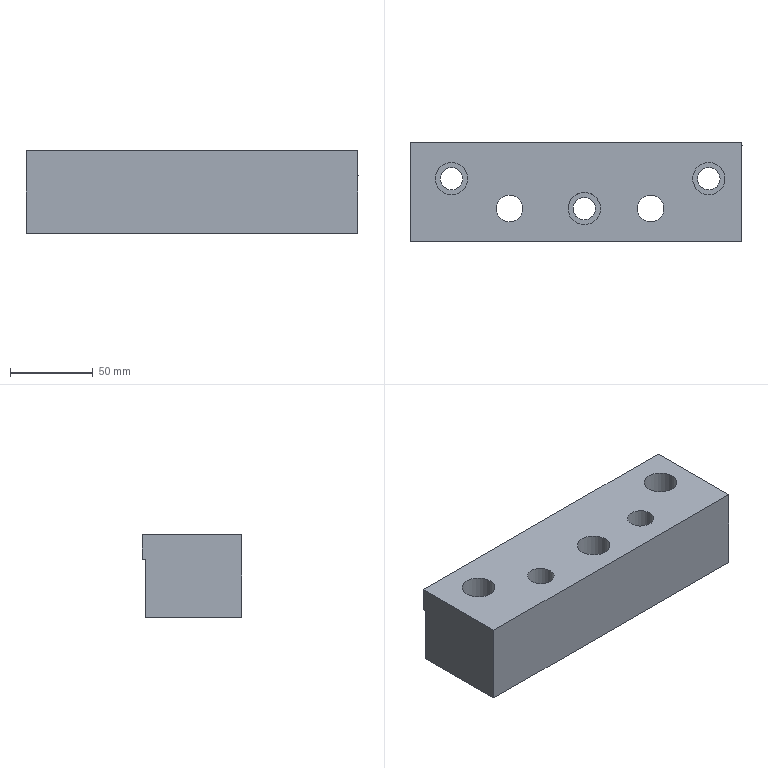Part | NX | features solid 2 | 1 solid | 19 faces | box 200 x 60.002 x 50 mm | volume 532750 mm3 | cylinder 8 | plane 7 | spline 4 | commonest cylinder face diameters 13.5 x3 19.5 x3 16 x2